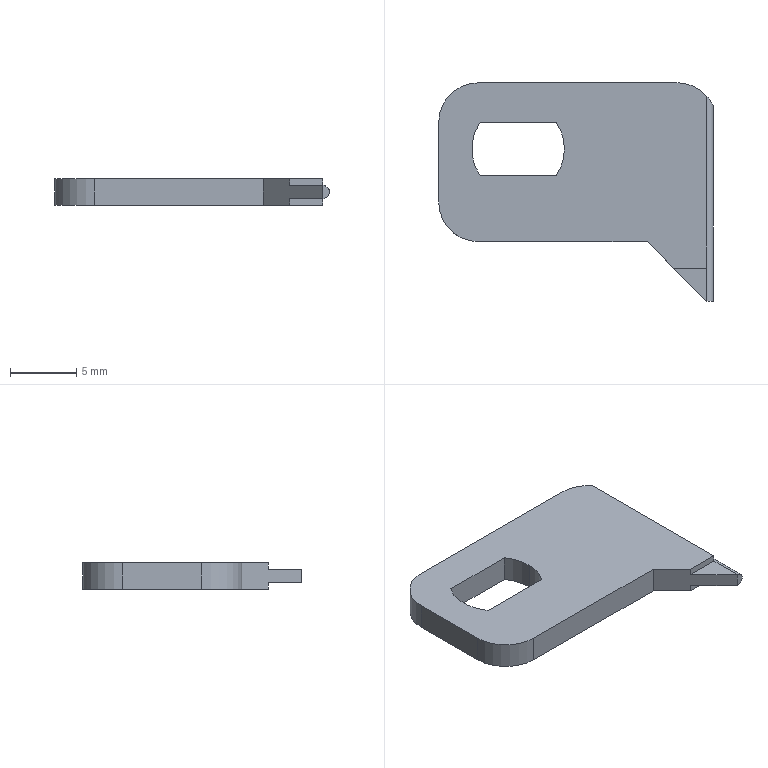Part | NX | 1 solid | 22 faces | box 20.75 x 16.5 x 2 mm | volume 447.181 mm3 | plane 15 | cylinder 7 | commonest cylinder face diameters 6 x3 7 x3 1 x1
STEP:
#1=CARTESIAN_POINT('',(14.25,3.984,0.));
#2=VERTEX_POINT('',#1);
#3=CARTESIAN_POINT('',(12.,5.,0.));
#4=VERTEX_POINT('',#3);
#5=CARTESIAN_POINT('',(12.,2.,0.));
#6=DIRECTION('',(0.,0.,1.));
#7=DIRECTION('',(0.75,0.6614,0.));
#8=AXIS2_PLACEMENT_3D('',#5,#6,#7);
#9=CIRCLE('',#8,3.);
#10=EDGE_CURVE('',#2,#4,#9,.T.);
#11=ORIENTED_EDGE('',*,*,#10,.F.);
#12=CARTESIAN_POINT('',(14.25,-9.,0.));
#13=VERTEX_POINT('',#12);
#14=CARTESIAN_POINT('',(14.25,3.984,0.));
#15=DIRECTION('',(0.,-1.,0.));
#16=VECTOR('',#15,1000.);
#17=LINE('',#14,#16);
#18=EDGE_CURVE('',#2,#13,#17,.T.);
#19=ORIENTED_EDGE('',*,*,#18,.T.);
#20=CARTESIAN_POINT('',(11.75,-9.,0.));
#21=VERTEX_POINT('',#20);
#22=CARTESIAN_POINT('',(14.25,-9.,0.));
#23=DIRECTION('',(-1.,0.,0.));
#24=VECTOR('',#23,1000.);
#25=LINE('',#22,#24);
#26=EDGE_CURVE('',#13,#21,#25,.T.);
#27=ORIENTED_EDGE('',*,*,#26,.T.);
#28=CARTESIAN_POINT('',(9.75,-7.,0.));
#29=VERTEX_POINT('',#28);
#30=CARTESIAN_POINT('',(9.75,-7.,0.));
#31=DIRECTION('',(0.7071,-0.7071,0.));
#32=VECTOR('',#31,1000.);
#33=LINE('',#30,#32);
#34=EDGE_CURVE('',#29,#21,#33,.T.);
#35=ORIENTED_EDGE('',*,*,#34,.F.);
#36=CARTESIAN_POINT('',(-3.,-7.,0.));
#37=VERTEX_POINT('',#36);
#38=CARTESIAN_POINT('',(9.75,-7.,0.));
#39=DIRECTION('',(-1.,0.,0.));
#40=VECTOR('',#39,1000.);
#41=LINE('',#38,#40);
#42=EDGE_CURVE('',#29,#37,#41,.T.);
#43=ORIENTED_EDGE('',*,*,#42,.T.);
#44=CARTESIAN_POINT('',(-6.,-4.,0.));
#45=VERTEX_POINT('',#44);
#46=CARTESIAN_POINT('',(-3.,-4.,0.));
#47=DIRECTION('',(0.,0.,1.));
#48=DIRECTION('',(-1.,0.,0.));
#49=AXIS2_PLACEMENT_3D('',#46,#47,#48);
#50=CIRCLE('',#49,3.);
#51=EDGE_CURVE('',#45,#37,#50,.T.);
#52=ORIENTED_EDGE('',*,*,#51,.F.);
#53=CARTESIAN_POINT('',(-6.,2.,0.));
#54=VERTEX_POINT('',#53);
#55=CARTESIAN_POINT('',(-6.,-4.,0.));
#56=DIRECTION('',(0.,1.,0.));
#57=VECTOR('',#56,1000.);
#58=LINE('',#55,#57);
#59=EDGE_CURVE('',#45,#54,#58,.T.);
#60=ORIENTED_EDGE('',*,*,#59,.T.);
#61=CARTESIAN_POINT('',(-3.,5.,0.));
#62=VERTEX_POINT('',#61);
#63=CARTESIAN_POINT('',(-3.,2.,0.));
#64=DIRECTION('',(0.,0.,1.));
#65=DIRECTION('',(0.,1.,0.));
#66=AXIS2_PLACEMENT_3D('',#63,#64,#65);
#67=CIRCLE('',#66,3.);
#68=EDGE_CURVE('',#62,#54,#67,.T.);
#69=ORIENTED_EDGE('',*,*,#68,.F.);
#70=CARTESIAN_POINT('',(-3.,5.,0.));
#71=DIRECTION('',(1.,0.,0.));
#72=VECTOR('',#71,1000.);
#73=LINE('',#70,#72);
#74=EDGE_CURVE('',#62,#4,#73,.T.);
#75=ORIENTED_EDGE('',*,*,#74,.T.);
#76=EDGE_LOOP('',(#11,#19,#27,#35,#43,#52,#60,#69,#75));
#77=FACE_BOUND('',#76,.T.);
#78=CARTESIAN_POINT('',(-2.872,-2.,0.));
#79=VERTEX_POINT('',#78);
#80=CARTESIAN_POINT('',(-2.872,2.,0.));
#81=VERTEX_POINT('',#80);
#82=CARTESIAN_POINT('',(0.,0.,0.));
#83=DIRECTION('',(0.,0.,-1.));
#84=DIRECTION('',(-1.,0.,0.));
#85=AXIS2_PLACEMENT_3D('',#82,#83,#84);
#86=CIRCLE('',#85,3.5);
#87=EDGE_CURVE('',#79,#81,#86,.T.);
#88=ORIENTED_EDGE('',*,*,#87,.F.);
#89=CARTESIAN_POINT('',(2.872,-2.,0.));
#90=VERTEX_POINT('',#89);
#91=CARTESIAN_POINT('',(-2.872,-2.,0.));
#92=DIRECTION('',(1.,0.,0.));
#93=VECTOR('',#92,1000.);
#94=LINE('',#91,#93);
#95=EDGE_CURVE('',#79,#90,#94,.T.);
#96=ORIENTED_EDGE('',*,*,#95,.T.);
#97=CARTESIAN_POINT('',(3.5,0.,0.));
#98=VERTEX_POINT('',#97);
#99=CARTESIAN_POINT('',(0.,0.,0.));
#100=DIRECTION('',(0.,0.,-1.));
#101=DIRECTION('',(1.,0.,0.));
#102=AXIS2_PLACEMENT_3D('',#99,#100,#101);
#103=CIRCLE('',#102,3.5);
#104=EDGE_CURVE('',#98,#90,#103,.T.);
#105=ORIENTED_EDGE('',*,*,#104,.F.);
#106=CARTESIAN_POINT('',(2.872,2.,0.));
#107=VERTEX_POINT('',#106);
#108=CARTESIAN_POINT('',(0.,0.,0.));
#109=DIRECTION('',(0.,0.,-1.));
#110=DIRECTION('',(1.,0.,0.));
#111=AXIS2_PLACEMENT_3D('',#108,#109,#110);
#112=CIRCLE('',#111,3.5);
#113=EDGE_CURVE('',#107,#98,#112,.T.);
#114=ORIENTED_EDGE('',*,*,#113,.F.);
#115=CARTESIAN_POINT('',(2.872,2.,0.));
#116=DIRECTION('',(-1.,0.,0.));
#117=VECTOR('',#116,1000.);
#118=LINE('',#115,#117);
#119=EDGE_CURVE('',#107,#81,#118,.T.);
#120=ORIENTED_EDGE('',*,*,#119,.T.);
#121=EDGE_LOOP('',(#88,#96,#105,#114,#120));
#122=FACE_BOUND('',#121,.T.);
#123=CARTESIAN_POINT('',(0.,0.,0.));
#124=DIRECTION('',(0.,0.,1.));
#125=DIRECTION('',(1.,0.,0.));
#126=AXIS2_PLACEMENT_3D('',#123,#124,#125);
#127=PLANE('',#126);
#128=ADVANCED_FACE('',(#77,#122),#127,.F.);
#129=ORIENTED_EDGE('',*,*,#10,.T.);
#130=CARTESIAN_POINT('',(12.,5.,2.));
#131=VERTEX_POINT('',#130);
#132=CARTESIAN_POINT('',(12.,5.,2.));
#133=DIRECTION('',(0.,0.,-1.));
#134=VECTOR('',#133,1000.);
#135=LINE('',#132,#134);
#136=EDGE_CURVE('',#131,#4,#135,.T.);
#137=ORIENTED_EDGE('',*,*,#136,.F.);
#138=CARTESIAN_POINT('',(14.25,3.984,2.));
#139=VERTEX_POINT('',#138);
#140=CARTESIAN_POINT('',(12.,2.,2.));
#141=DIRECTION('',(0.,0.,-1.));
#142=DIRECTION('',(0.,1.,0.));
#143=AXIS2_PLACEMENT_3D('',#140,#141,#142);
#144=CIRCLE('',#143,3.);
#145=EDGE_CURVE('',#131,#139,#144,.T.);
#146=ORIENTED_EDGE('',*,*,#145,.T.);
#147=CARTESIAN_POINT('',(14.25,3.984,1.5));
#148=VERTEX_POINT('',#147);
#149=CARTESIAN_POINT('',(14.25,3.984,1.5));
#150=DIRECTION('',(0.,0.,1.));
#151=VECTOR('',#150,1000.);
#152=LINE('',#149,#151);
#153=EDGE_CURVE('',#148,#139,#152,.T.);
#154=ORIENTED_EDGE('',*,*,#153,.F.);
#155=CARTESIAN_POINT('',(14.25,3.984,0.5));
#156=VERTEX_POINT('',#155);
#157=CARTESIAN_POINT('',(14.25,3.984,1.5));
#158=CARTESIAN_POINT('',(14.346,3.875,1.5));
#159=CARTESIAN_POINT('',(14.546,3.604,1.43));
#160=CARTESIAN_POINT('',(14.718,3.281,1.228));
#161=CARTESIAN_POINT('',(14.772,3.144,0.9992));
#162=CARTESIAN_POINT('',(14.717,3.282,0.7707));
#163=CARTESIAN_POINT('',(14.546,3.604,0.5699));
#164=CARTESIAN_POINT('',(14.346,3.875,0.5));
#165=CARTESIAN_POINT('',(14.25,3.984,0.5));
#166=B_SPLINE_CURVE_WITH_KNOTS('',3,(#157,#158,#159,#160,#161,#162,#163,#164,#165),.UNSPECIFIED.,.F.,.F.,(4,1,1,1,1,1,4),(0.,0.125,0.25,0.5,0.75,0.875,1.),.UNSPECIFIED.);
#167=EDGE_CURVE('',#156,#148,#166,.F.);
#168=ORIENTED_EDGE('',*,*,#167,.F.);
#169=CARTESIAN_POINT('',(14.25,3.984,0.));
#170=DIRECTION('',(0.,0.,1.));
#171=VECTOR('',#170,1000.);
#172=LINE('',#169,#171);
#173=EDGE_CURVE('',#2,#156,#172,.T.);
#174=ORIENTED_EDGE('',*,*,#173,.F.);
#175=EDGE_LOOP('',(#129,#137,#146,#154,#168,#174));
#176=FACE_BOUND('',#175,.T.);
#177=CARTESIAN_POINT('',(12.,2.,0.));
#178=DIRECTION('',(0.,0.,1.));
#179=DIRECTION('',(1.,0.,0.));
#180=AXIS2_PLACEMENT_3D('',#177,#178,#179);
#181=CYLINDRICAL_SURFACE('',#180,3.);
#182=ADVANCED_FACE('',(#176),#181,.T.);
#183=ORIENTED_EDGE('',*,*,#18,.F.);
#184=ORIENTED_EDGE('',*,*,#173,.T.);
#185=CARTESIAN_POINT('',(14.25,-9.,0.5));
#186=VERTEX_POINT('',#185);
#187=CARTESIAN_POINT('',(14.25,-11.5,0.5));
#188=DIRECTION('',(0.,-1.,0.));
#189=VECTOR('',#188,1000.);
#190=LINE('',#187,#189);
#191=EDGE_CURVE('',#156,#186,#190,.T.);
#192=ORIENTED_EDGE('',*,*,#191,.T.);
#193=CARTESIAN_POINT('',(14.25,-9.,0.5));
#194=DIRECTION('',(0.,0.,-1.));
#195=VECTOR('',#194,1000.);
#196=LINE('',#193,#195);
#197=EDGE_CURVE('',#186,#13,#196,.T.);
#198=ORIENTED_EDGE('',*,*,#197,.T.);
#199=EDGE_LOOP('',(#183,#184,#192,#198));
#200=FACE_BOUND('',#199,.T.);
#201=CARTESIAN_POINT('',(14.25,-11.5,0.5));
#202=DIRECTION('',(-1.,0.,0.));
#203=DIRECTION('',(0.,0.,1.));
#204=AXIS2_PLACEMENT_3D('',#201,#202,#203);
#205=PLANE('',#204);
#206=ADVANCED_FACE('',(#200),#205,.F.);
#207=ORIENTED_EDGE('',*,*,#26,.F.);
#208=ORIENTED_EDGE('',*,*,#197,.F.);
#209=CARTESIAN_POINT('',(11.75,-9.,0.5));
#210=VERTEX_POINT('',#209);
#211=CARTESIAN_POINT('',(11.75,-9.,0.5));
#212=DIRECTION('',(1.,0.,0.));
#213=VECTOR('',#212,1000.);
#214=LINE('',#211,#213);
#215=EDGE_CURVE('',#210,#186,#214,.T.);
#216=ORIENTED_EDGE('',*,*,#215,.F.);
#217=CARTESIAN_POINT('',(11.75,-9.,0.5));
#218=DIRECTION('',(0.,0.,-1.));
#219=VECTOR('',#218,1000.);
#220=LINE('',#217,#219);
#221=EDGE_CURVE('',#210,#21,#220,.T.);
#222=ORIENTED_EDGE('',*,*,#221,.T.);
#223=EDGE_LOOP('',(#207,#208,#216,#222));
#224=FACE_BOUND('',#223,.T.);
#225=CARTESIAN_POINT('',(15.,-9.,0.));
#226=DIRECTION('',(0.,1.,0.));
#227=DIRECTION('',(1.,0.,0.));
#228=AXIS2_PLACEMENT_3D('',#225,#226,#227);
#229=PLANE('',#228);
#230=ADVANCED_FACE('',(#224),#229,.F.);
#231=CARTESIAN_POINT('',(14.25,-11.5,0.5));
#232=VERTEX_POINT('',#231);
#233=CARTESIAN_POINT('',(11.75,-9.,0.5));
#234=DIRECTION('',(0.7071,-0.7071,0.));
#235=VECTOR('',#234,1000.);
#236=LINE('',#233,#235);
#237=EDGE_CURVE('',#210,#232,#236,.T.);
#238=ORIENTED_EDGE('',*,*,#237,.T.);
#239=CARTESIAN_POINT('',(14.25,-11.5,1.5));
#240=VERTEX_POINT('',#239);
#241=CARTESIAN_POINT('',(14.25,-11.5,1.5));
#242=DIRECTION('',(0.,0.,-1.));
#243=VECTOR('',#242,1000.);
#244=LINE('',#241,#243);
#245=EDGE_CURVE('',#240,#232,#244,.T.);
#246=ORIENTED_EDGE('',*,*,#245,.F.);
#247=CARTESIAN_POINT('',(11.75,-9.,1.5));
#248=VERTEX_POINT('',#247);
#249=CARTESIAN_POINT('',(14.25,-11.5,1.5));
#250=DIRECTION('',(-0.7071,0.7071,0.));
#251=VECTOR('',#250,1000.);
#252=LINE('',#249,#251);
#253=EDGE_CURVE('',#240,#248,#252,.T.);
#254=ORIENTED_EDGE('',*,*,#253,.T.);
#255=CARTESIAN_POINT('',(11.75,-9.,2.));
#256=VERTEX_POINT('',#255);
#257=CARTESIAN_POINT('',(11.75,-9.,1.5));
#258=DIRECTION('',(0.,0.,1.));
#259=VECTOR('',#258,1000.);
#260=LINE('',#257,#259);
#261=EDGE_CURVE('',#248,#256,#260,.T.);
#262=ORIENTED_EDGE('',*,*,#261,.T.);
#263=CARTESIAN_POINT('',(9.75,-7.,2.));
#264=VERTEX_POINT('',#263);
#265=CARTESIAN_POINT('',(11.75,-9.,2.));
#266=DIRECTION('',(-0.7071,0.7071,0.));
#267=VECTOR('',#266,1000.);
#268=LINE('',#265,#267);
#269=EDGE_CURVE('',#256,#264,#268,.T.);
#270=ORIENTED_EDGE('',*,*,#269,.T.);
#271=CARTESIAN_POINT('',(9.75,-7.,2.));
#272=DIRECTION('',(0.,0.,-1.));
#273=VECTOR('',#272,1000.);
#274=LINE('',#271,#273);
#275=EDGE_CURVE('',#264,#29,#274,.T.);
#276=ORIENTED_EDGE('',*,*,#275,.T.);
#277=ORIENTED_EDGE('',*,*,#34,.T.);
#278=ORIENTED_EDGE('',*,*,#221,.F.);
#279=EDGE_LOOP('',(#238,#246,#254,#262,#270,#276,#277,#278));
#280=FACE_BOUND('',#279,.T.);
#281=CARTESIAN_POINT('',(9.75,-7.,0.));
#282=DIRECTION('',(-0.7071,-0.7071,0.));
#283=DIRECTION('',(-0.7071,0.7071,0.));
#284=AXIS2_PLACEMENT_3D('',#281,#282,#283);
#285=PLANE('',#284);
#286=ADVANCED_FACE('',(#280),#285,.T.);
#287=ORIENTED_EDGE('',*,*,#215,.T.);
#288=CARTESIAN_POINT('',(14.25,-11.5,0.5));
#289=DIRECTION('',(0.,-1.,0.));
#290=VECTOR('',#289,1000.);
#291=LINE('',#288,#290);
#292=EDGE_CURVE('',#186,#232,#291,.T.);
#293=ORIENTED_EDGE('',*,*,#292,.T.);
#294=ORIENTED_EDGE('',*,*,#237,.F.);
#295=EDGE_LOOP('',(#287,#293,#294));
#296=FACE_BOUND('',#295,.T.);
#297=CARTESIAN_POINT('',(15.,-9.,0.5));
#298=DIRECTION('',(0.,0.,1.));
#299=DIRECTION('',(1.,0.,0.));
#300=AXIS2_PLACEMENT_3D('',#297,#298,#299);
#301=PLANE('',#300);
#302=ADVANCED_FACE('',(#296),#301,.F.);
#303=CARTESIAN_POINT('',(14.25,-11.5,1.));
#304=DIRECTION('',(0.,1.,0.));
#305=DIRECTION('',(0.,0.,1.));
#306=AXIS2_PLACEMENT_3D('',#303,#304,#305);
#307=CIRCLE('',#306,0.5);
#308=EDGE_CURVE('',#240,#232,#307,.T.);
#309=ORIENTED_EDGE('',*,*,#308,.T.);
#310=ORIENTED_EDGE('',*,*,#292,.F.);
#311=ORIENTED_EDGE('',*,*,#191,.F.);
#312=ORIENTED_EDGE('',*,*,#167,.T.);
#313=CARTESIAN_POINT('',(14.25,-9.,1.5));
#314=VERTEX_POINT('',#313);
#315=CARTESIAN_POINT('',(14.25,-11.5,1.5));
#316=DIRECTION('',(0.,-1.,0.));
#317=VECTOR('',#316,1000.);
#318=LINE('',#315,#317);
#319=EDGE_CURVE('',#148,#314,#318,.T.);
#320=ORIENTED_EDGE('',*,*,#319,.T.);
#321=CARTESIAN_POINT('',(14.25,-11.5,1.5));
#322=DIRECTION('',(0.,-1.,0.));
#323=VECTOR('',#322,1000.);
#324=LINE('',#321,#323);
#325=EDGE_CURVE('',#314,#240,#324,.T.);
#326=ORIENTED_EDGE('',*,*,#325,.T.);
#327=EDGE_LOOP('',(#309,#310,#311,#312,#320,#326));
#328=FACE_BOUND('',#327,.T.);
#329=CARTESIAN_POINT('',(14.25,-11.5,1.));
#330=DIRECTION('',(0.,-1.,0.));
#331=DIRECTION('',(0.,0.,-1.));
#332=AXIS2_PLACEMENT_3D('',#329,#330,#331);
#333=CYLINDRICAL_SURFACE('',#332,0.5);
#334=ADVANCED_FACE('',(#328),#333,.T.);
#335=ORIENTED_EDGE('',*,*,#308,.F.);
#336=ORIENTED_EDGE('',*,*,#245,.T.);
#337=EDGE_LOOP('',(#335,#336));
#338=FACE_BOUND('',#337,.T.);
#339=CARTESIAN_POINT('',(14.25,-11.5,0.));
#340=DIRECTION('',(0.,-1.,0.));
#341=DIRECTION('',(0.,0.,-1.));
#342=AXIS2_PLACEMENT_3D('',#339,#340,#341);
#343=PLANE('',#342);
#344=ADVANCED_FACE('',(#338),#343,.T.);
#345=CARTESIAN_POINT('',(11.75,-9.,1.5));
#346=DIRECTION('',(1.,0.,0.));
#347=VECTOR('',#346,1000.);
#348=LINE('',#345,#347);
#349=EDGE_CURVE('',#248,#314,#348,.T.);
#350=ORIENTED_EDGE('',*,*,#349,.F.);
#351=ORIENTED_EDGE('',*,*,#253,.F.);
#352=ORIENTED_EDGE('',*,*,#325,.F.);
#353=EDGE_LOOP('',(#350,#351,#352));
#354=FACE_BOUND('',#353,.T.);
#355=CARTESIAN_POINT('',(15.,-11.5,1.5));
#356=DIRECTION('',(0.,0.,-1.));
#357=DIRECTION('',(0.,-1.,0.));
#358=AXIS2_PLACEMENT_3D('',#355,#356,#357);
#359=PLANE('',#358);
#360=ADVANCED_FACE('',(#354),#359,.F.);
#361=CARTESIAN_POINT('',(14.25,-9.,2.));
#362=VERTEX_POINT('',#361);
#363=CARTESIAN_POINT('',(14.25,-9.,2.));
#364=DIRECTION('',(-1.,0.,0.));
#365=VECTOR('',#364,1000.);
#366=LINE('',#363,#365);
#367=EDGE_CURVE('',#362,#256,#366,.T.);
#368=ORIENTED_EDGE('',*,*,#367,.T.);
#369=ORIENTED_EDGE('',*,*,#261,.F.);
#370=ORIENTED_EDGE('',*,*,#349,.T.);
#371=CARTESIAN_POINT('',(14.25,-9.,2.));
#372=DIRECTION('',(0.,0.,-1.));
#373=VECTOR('',#372,1000.);
#374=LINE('',#371,#373);
#375=EDGE_CURVE('',#362,#314,#374,.T.);
#376=ORIENTED_EDGE('',*,*,#375,.F.);
#377=EDGE_LOOP('',(#368,#369,#370,#376));
#378=FACE_BOUND('',#377,.T.);
#379=CARTESIAN_POINT('',(15.,-9.,1.5));
#380=DIRECTION('',(0.,1.,0.));
#381=DIRECTION('',(1.,0.,0.));
#382=AXIS2_PLACEMENT_3D('',#379,#380,#381);
#383=PLANE('',#382);
#384=ADVANCED_FACE('',(#378),#383,.F.);
#385=ORIENTED_EDGE('',*,*,#145,.F.);
#386=CARTESIAN_POINT('',(-3.,5.,2.));
#387=VERTEX_POINT('',#386);
#388=CARTESIAN_POINT('',(-3.,5.,2.));
#389=DIRECTION('',(1.,0.,0.));
#390=VECTOR('',#389,1000.);
#391=LINE('',#388,#390);
#392=EDGE_CURVE('',#387,#131,#391,.T.);
#393=ORIENTED_EDGE('',*,*,#392,.F.);
#394=CARTESIAN_POINT('',(-6.,2.,2.));
#395=VERTEX_POINT('',#394);
#396=CARTESIAN_POINT('',(-3.,2.,2.));
#397=DIRECTION('',(0.,0.,-1.));
#398=DIRECTION('',(-1.,0.,0.));
#399=AXIS2_PLACEMENT_3D('',#396,#397,#398);
#400=CIRCLE('',#399,3.);
#401=EDGE_CURVE('',#395,#387,#400,.T.);
#402=ORIENTED_EDGE('',*,*,#401,.F.);
#403=CARTESIAN_POINT('',(-6.,-4.,2.));
#404=VERTEX_POINT('',#403);
#405=CARTESIAN_POINT('',(-6.,-4.,2.));
#406=DIRECTION('',(0.,1.,0.));
#407=VECTOR('',#406,1000.);
#408=LINE('',#405,#407);
#409=EDGE_CURVE('',#404,#395,#408,.T.);
#410=ORIENTED_EDGE('',*,*,#409,.F.);
#411=CARTESIAN_POINT('',(-3.,-7.,2.));
#412=VERTEX_POINT('',#411);
#413=CARTESIAN_POINT('',(-3.,-4.,2.));
#414=DIRECTION('',(0.,0.,-1.));
#415=DIRECTION('',(0.,-1.,0.));
#416=AXIS2_PLACEMENT_3D('',#413,#414,#415);
#417=CIRCLE('',#416,3.);
#418=EDGE_CURVE('',#412,#404,#417,.T.);
#419=ORIENTED_EDGE('',*,*,#418,.F.);
#420=CARTESIAN_POINT('',(9.75,-7.,2.));
#421=DIRECTION('',(-1.,0.,0.));
#422=VECTOR('',#421,1000.);
#423=LINE('',#420,#422);
#424=EDGE_CURVE('',#264,#412,#423,.T.);
#425=ORIENTED_EDGE('',*,*,#424,.F.);
#426=ORIENTED_EDGE('',*,*,#269,.F.);
#427=ORIENTED_EDGE('',*,*,#367,.F.);
#428=CARTESIAN_POINT('',(14.25,3.984,2.));
#429=DIRECTION('',(0.,-1.,0.));
#430=VECTOR('',#429,1000.);
#431=LINE('',#428,#430);
#432=EDGE_CURVE('',#139,#362,#431,.T.);
#433=ORIENTED_EDGE('',*,*,#432,.F.);
#434=EDGE_LOOP('',(#385,#393,#402,#410,#419,#425,#426,#427,#433));
#435=FACE_BOUND('',#434,.T.);
#436=CARTESIAN_POINT('',(-2.872,2.,2.));
#437=VERTEX_POINT('',#436);
#438=CARTESIAN_POINT('',(-2.872,-2.,2.));
#439=VERTEX_POINT('',#438);
#440=CARTESIAN_POINT('',(0.,0.,2.));
#441=DIRECTION('',(0.,0.,1.));
#442=DIRECTION('',(-1.,0.,0.));
#443=AXIS2_PLACEMENT_3D('',#440,#441,#442);
#444=CIRCLE('',#443,3.5);
#445=EDGE_CURVE('',#437,#439,#444,.T.);
#446=ORIENTED_EDGE('',*,*,#445,.F.);
#447=CARTESIAN_POINT('',(2.872,2.,2.));
#448=VERTEX_POINT('',#447);
#449=CARTESIAN_POINT('',(2.872,2.,2.));
#450=DIRECTION('',(-1.,0.,0.));
#451=VECTOR('',#450,1000.);
#452=LINE('',#449,#451);
#453=EDGE_CURVE('',#448,#437,#452,.T.);
#454=ORIENTED_EDGE('',*,*,#453,.F.);
#455=CARTESIAN_POINT('',(3.5,0.,2.));
#456=VERTEX_POINT('',#455);
#457=CARTESIAN_POINT('',(0.,0.,2.));
#458=DIRECTION('',(0.,0.,1.));
#459=DIRECTION('',(1.,0.,0.));
#460=AXIS2_PLACEMENT_3D('',#457,#458,#459);
#461=CIRCLE('',#460,3.5);
#462=EDGE_CURVE('',#456,#448,#461,.T.);
#463=ORIENTED_EDGE('',*,*,#462,.F.);
#464=CARTESIAN_POINT('',(2.872,-2.,2.));
#465=VERTEX_POINT('',#464);
#466=CARTESIAN_POINT('',(0.,0.,2.));
#467=DIRECTION('',(0.,0.,1.));
#468=DIRECTION('',(1.,0.,0.));
#469=AXIS2_PLACEMENT_3D('',#466,#467,#468);
#470=CIRCLE('',#469,3.5);
#471=EDGE_CURVE('',#465,#456,#470,.T.);
#472=ORIENTED_EDGE('',*,*,#471,.F.);
#473=CARTESIAN_POINT('',(-2.872,-2.,2.));
#474=DIRECTION('',(1.,0.,0.));
#475=VECTOR('',#474,1000.);
#476=LINE('',#473,#475);
#477=EDGE_CURVE('',#439,#465,#476,.T.);
#478=ORIENTED_EDGE('',*,*,#477,.F.);
#479=EDGE_LOOP('',(#446,#454,#463,#472,#478));
#480=FACE_BOUND('',#479,.T.);
#481=CARTESIAN_POINT('',(0.,0.,2.));
#482=DIRECTION('',(0.,0.,1.));
#483=DIRECTION('',(1.,0.,0.));
#484=AXIS2_PLACEMENT_3D('',#481,#482,#483);
#485=PLANE('',#484);
#486=ADVANCED_FACE('',(#435,#480),#485,.T.);
#487=ORIENTED_EDGE('',*,*,#432,.T.);
#488=ORIENTED_EDGE('',*,*,#375,.T.);
#489=ORIENTED_EDGE('',*,*,#319,.F.);
#490=ORIENTED_EDGE('',*,*,#153,.T.);
#491=EDGE_LOOP('',(#487,#488,#489,#490));
#492=FACE_BOUND('',#491,.T.);
#493=CARTESIAN_POINT('',(14.25,-11.5,2.));
#494=DIRECTION('',(-1.,0.,0.));
#495=DIRECTION('',(0.,0.,1.));
#496=AXIS2_PLACEMENT_3D('',#493,#494,#495);
#497=PLANE('',#496);
#498=ADVANCED_FACE('',(#492),#497,.F.);
#499=ORIENTED_EDGE('',*,*,#42,.F.);
#500=ORIENTED_EDGE('',*,*,#275,.F.);
#501=ORIENTED_EDGE('',*,*,#424,.T.);
#502=CARTESIAN_POINT('',(-3.,-7.,2.));
#503=DIRECTION('',(0.,0.,-1.));
#504=VECTOR('',#503,1000.);
#505=LINE('',#502,#504);
#506=EDGE_CURVE('',#412,#37,#505,.T.);
#507=ORIENTED_EDGE('',*,*,#506,.T.);
#508=EDGE_LOOP('',(#499,#500,#501,#507));
#509=FACE_BOUND('',#508,.T.);
#510=CARTESIAN_POINT('',(-3.,-7.,0.));
#511=DIRECTION('',(0.,-1.,0.));
#512=DIRECTION('',(0.,0.,-1.));
#513=AXIS2_PLACEMENT_3D('',#510,#511,#512);
#514=PLANE('',#513);
#515=ADVANCED_FACE('',(#509),#514,.T.);
#516=ORIENTED_EDGE('',*,*,#51,.T.);
#517=ORIENTED_EDGE('',*,*,#506,.F.);
#518=ORIENTED_EDGE('',*,*,#418,.T.);
#519=CARTESIAN_POINT('',(-6.,-4.,0.));
#520=DIRECTION('',(0.,0.,1.));
#521=VECTOR('',#520,1000.);
#522=LINE('',#519,#521);
#523=EDGE_CURVE('',#45,#404,#522,.T.);
#524=ORIENTED_EDGE('',*,*,#523,.F.);
#525=EDGE_LOOP('',(#516,#517,#518,#524));
#526=FACE_BOUND('',#525,.T.);
#527=CARTESIAN_POINT('',(-3.,-4.,0.));
#528=DIRECTION('',(0.,0.,1.));
#529=DIRECTION('',(1.,0.,0.));
#530=AXIS2_PLACEMENT_3D('',#527,#528,#529);
#531=CYLINDRICAL_SURFACE('',#530,3.);
#532=ADVANCED_FACE('',(#526),#531,.T.);
#533=ORIENTED_EDGE('',*,*,#59,.F.);
#534=ORIENTED_EDGE('',*,*,#523,.T.);
#535=ORIENTED_EDGE('',*,*,#409,.T.);
#536=CARTESIAN_POINT('',(-6.,2.,0.));
#537=DIRECTION('',(0.,0.,1.));
#538=VECTOR('',#537,1000.);
#539=LINE('',#536,#538);
#540=EDGE_CURVE('',#54,#395,#539,.T.);
#541=ORIENTED_EDGE('',*,*,#540,.F.);
#542=EDGE_LOOP('',(#533,#534,#535,#541));
#543=FACE_BOUND('',#542,.T.);
#544=CARTESIAN_POINT('',(-6.,2.,0.));
#545=DIRECTION('',(-1.,0.,0.));
#546=DIRECTION('',(0.,0.,1.));
#547=AXIS2_PLACEMENT_3D('',#544,#545,#546);
#548=PLANE('',#547);
#549=ADVANCED_FACE('',(#543),#548,.T.);
#550=ORIENTED_EDGE('',*,*,#68,.T.);
#551=ORIENTED_EDGE('',*,*,#540,.T.);
#552=ORIENTED_EDGE('',*,*,#401,.T.);
#553=CARTESIAN_POINT('',(-3.,5.,0.));
#554=DIRECTION('',(0.,0.,1.));
#555=VECTOR('',#554,1000.);
#556=LINE('',#553,#555);
#557=EDGE_CURVE('',#62,#387,#556,.T.);
#558=ORIENTED_EDGE('',*,*,#557,.F.);
#559=EDGE_LOOP('',(#550,#551,#552,#558));
#560=FACE_BOUND('',#559,.T.);
#561=CARTESIAN_POINT('',(-3.,2.,0.));
#562=DIRECTION('',(0.,0.,1.));
#563=DIRECTION('',(1.,0.,0.));
#564=AXIS2_PLACEMENT_3D('',#561,#562,#563);
#565=CYLINDRICAL_SURFACE('',#564,3.);
#566=ADVANCED_FACE('',(#560),#565,.T.);
#567=ORIENTED_EDGE('',*,*,#74,.F.);
#568=ORIENTED_EDGE('',*,*,#557,.T.);
#569=ORIENTED_EDGE('',*,*,#392,.T.);
#570=ORIENTED_EDGE('',*,*,#136,.T.);
#571=EDGE_LOOP('',(#567,#568,#569,#570));
#572=FACE_BOUND('',#571,.T.);
#573=CARTESIAN_POINT('',(12.,5.,0.));
#574=DIRECTION('',(0.,1.,0.));
#575=DIRECTION('',(1.,0.,0.));
#576=AXIS2_PLACEMENT_3D('',#573,#574,#575);
#577=PLANE('',#576);
#578=ADVANCED_FACE('',(#572),#577,.T.);
#579=ORIENTED_EDGE('',*,*,#87,.T.);
#580=CARTESIAN_POINT('',(-2.872,2.,2.));
#581=DIRECTION('',(0.,0.,-1.));
#582=VECTOR('',#581,1000.);
#583=LINE('',#580,#582);
#584=EDGE_CURVE('',#437,#81,#583,.T.);
#585=ORIENTED_EDGE('',*,*,#584,.F.);
#586=ORIENTED_EDGE('',*,*,#445,.T.);
#587=CARTESIAN_POINT('',(-2.872,-2.,0.));
#588=DIRECTION('',(0.,0.,1.));
#589=VECTOR('',#588,1000.);
#590=LINE('',#587,#589);
#591=EDGE_CURVE('',#79,#439,#590,.T.);
#592=ORIENTED_EDGE('',*,*,#591,.F.);
#593=EDGE_LOOP('',(#579,#585,#586,#592));
#594=FACE_BOUND('',#593,.T.);
#595=CARTESIAN_POINT('',(0.,0.,0.));
#596=DIRECTION('',(0.,0.,1.));
#597=DIRECTION('',(1.,0.,0.));
#598=AXIS2_PLACEMENT_3D('',#595,#596,#597);
#599=CYLINDRICAL_SURFACE('',#598,3.5);
#600=ADVANCED_FACE('',(#594),#599,.F.);
#601=ORIENTED_EDGE('',*,*,#95,.F.);
#602=ORIENTED_EDGE('',*,*,#591,.T.);
#603=ORIENTED_EDGE('',*,*,#477,.T.);
#604=CARTESIAN_POINT('',(2.872,-2.,2.));
#605=DIRECTION('',(0.,0.,-1.));
#606=VECTOR('',#605,1000.);
#607=LINE('',#604,#606);
#608=EDGE_CURVE('',#465,#90,#607,.T.);
#609=ORIENTED_EDGE('',*,*,#608,.T.);
#610=EDGE_LOOP('',(#601,#602,#603,#609));
#611=FACE_BOUND('',#610,.T.);
#612=CARTESIAN_POINT('',(2.872,-2.,0.));
#613=DIRECTION('',(0.,1.,0.));
#614=DIRECTION('',(1.,0.,0.));
#615=AXIS2_PLACEMENT_3D('',#612,#613,#614);
#616=PLANE('',#615);
#617=ADVANCED_FACE('',(#611),#616,.T.);
#618=CARTESIAN_POINT('',(3.5,0.,0.));
#619=DIRECTION('',(0.,0.,1.));
#620=VECTOR('',#619,1000.);
#621=LINE('',#618,#620);
#622=EDGE_CURVE('',#98,#456,#621,.T.);
#623=ORIENTED_EDGE('',*,*,#622,.F.);
#624=ORIENTED_EDGE('',*,*,#104,.T.);
#625=ORIENTED_EDGE('',*,*,#608,.F.);
#626=ORIENTED_EDGE('',*,*,#471,.T.);
#627=EDGE_LOOP('',(#623,#624,#625,#626));
#628=FACE_BOUND('',#627,.T.);
#629=CARTESIAN_POINT('',(0.,0.,0.));
#630=DIRECTION('',(0.,0.,1.));
#631=DIRECTION('',(1.,0.,0.));
#632=AXIS2_PLACEMENT_3D('',#629,#630,#631);
#633=CYLINDRICAL_SURFACE('',#632,3.5);
#634=ADVANCED_FACE('',(#628),#633,.F.);
#635=ORIENTED_EDGE('',*,*,#119,.F.);
#636=CARTESIAN_POINT('',(2.872,2.,0.));
#637=DIRECTION('',(0.,0.,1.));
#638=VECTOR('',#637,1000.);
#639=LINE('',#636,#638);
#640=EDGE_CURVE('',#107,#448,#639,.T.);
#641=ORIENTED_EDGE('',*,*,#640,.T.);
#642=ORIENTED_EDGE('',*,*,#453,.T.);
#643=ORIENTED_EDGE('',*,*,#584,.T.);
#644=EDGE_LOOP('',(#635,#641,#642,#643));
#645=FACE_BOUND('',#644,.T.);
#646=CARTESIAN_POINT('',(-2.872,2.,0.));
#647=DIRECTION('',(0.,-1.,0.));
#648=DIRECTION('',(0.,0.,-1.));
#649=AXIS2_PLACEMENT_3D('',#646,#647,#648);
#650=PLANE('',#649);
#651=ADVANCED_FACE('',(#645),#650,.T.);
#652=ORIENTED_EDGE('',*,*,#113,.T.);
#653=ORIENTED_EDGE('',*,*,#622,.T.);
#654=ORIENTED_EDGE('',*,*,#462,.T.);
#655=ORIENTED_EDGE('',*,*,#640,.F.);
#656=EDGE_LOOP('',(#652,#653,#654,#655));
#657=FACE_BOUND('',#656,.T.);
#658=CARTESIAN_POINT('',(0.,0.,0.));
#659=DIRECTION('',(0.,0.,1.));
#660=DIRECTION('',(1.,0.,0.));
#661=AXIS2_PLACEMENT_3D('',#658,#659,#660);
#662=CYLINDRICAL_SURFACE('',#661,3.5);
#663=ADVANCED_FACE('',(#657),#662,.F.);
#664=CLOSED_SHELL('',(#128,#182,#206,#230,#286,#302,#334,#344,#360,#384,#486,#498,#515,#532,#549,#566,#578,#600,#617,#634,#651,#663));
#665=MANIFOLD_SOLID_BREP('',#664);
#666=(LENGTH_UNIT()NAMED_UNIT(*)SI_UNIT(.MILLI.,.METRE.));
#667=UNCERTAINTY_MEASURE_WITH_UNIT(LENGTH_MEASURE(0.0508),#666,'','');
#668=(NAMED_UNIT(*)PLANE_ANGLE_UNIT()SI_UNIT($,.RADIAN.));
#669=(NAMED_UNIT(*)SI_UNIT($,.STERADIAN.)SOLID_ANGLE_UNIT());
#670=(GEOMETRIC_REPRESENTATION_CONTEXT(3)GLOBAL_UNCERTAINTY_ASSIGNED_CONTEXT((#667))GLOBAL_UNIT_ASSIGNED_CONTEXT((#666,#668,#669))REPRESENTATION_CONTEXT('',''));
#671=ADVANCED_BREP_SHAPE_REPRESENTATION('',(#665),#670);